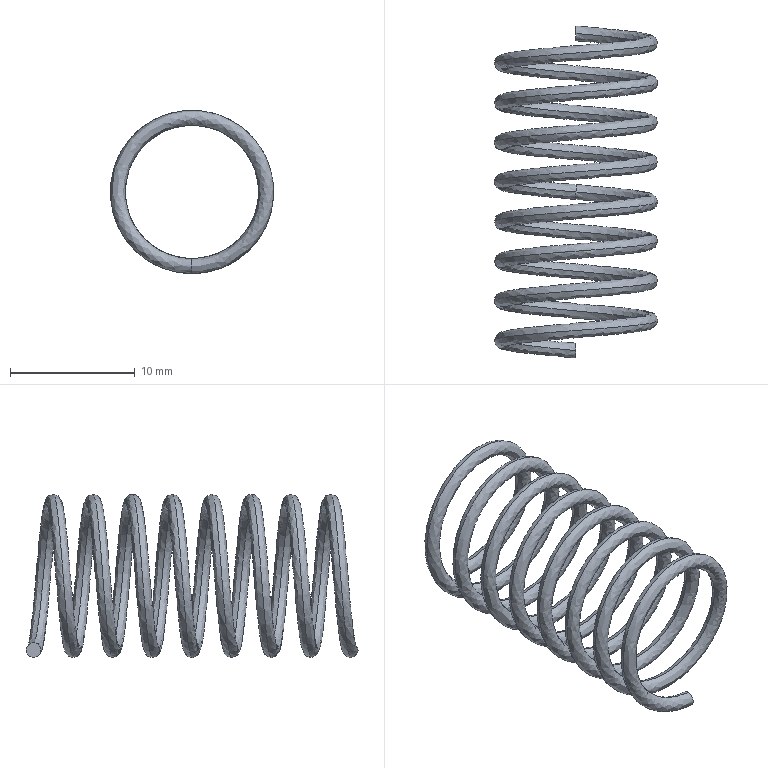Part | NX | features BREP 1 | 1 solid | 6 faces | box 13.081 x 26.594 x 13.081 mm | volume 333.972 mm3 | spline 4 | plane 2